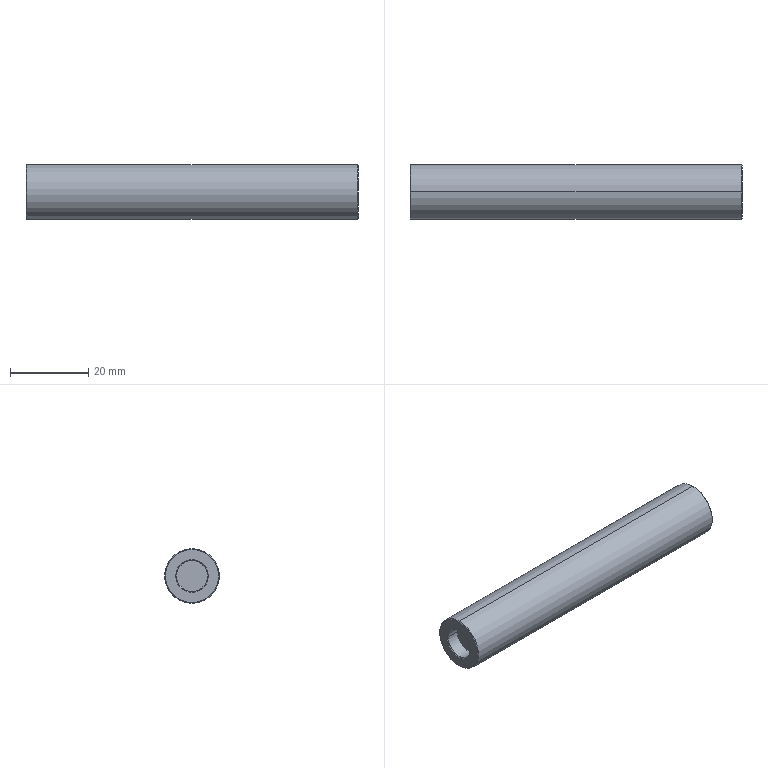Part | STEP file | 03-13 Suction column | 1 solid | 19 faces | box 85 x 14 x 14 mm | volume 12701 mm3 | cone 10 | cylinder 6 | plane 3 | commonest cylinder face diameters 4.2 x2 8 x2 14 x2